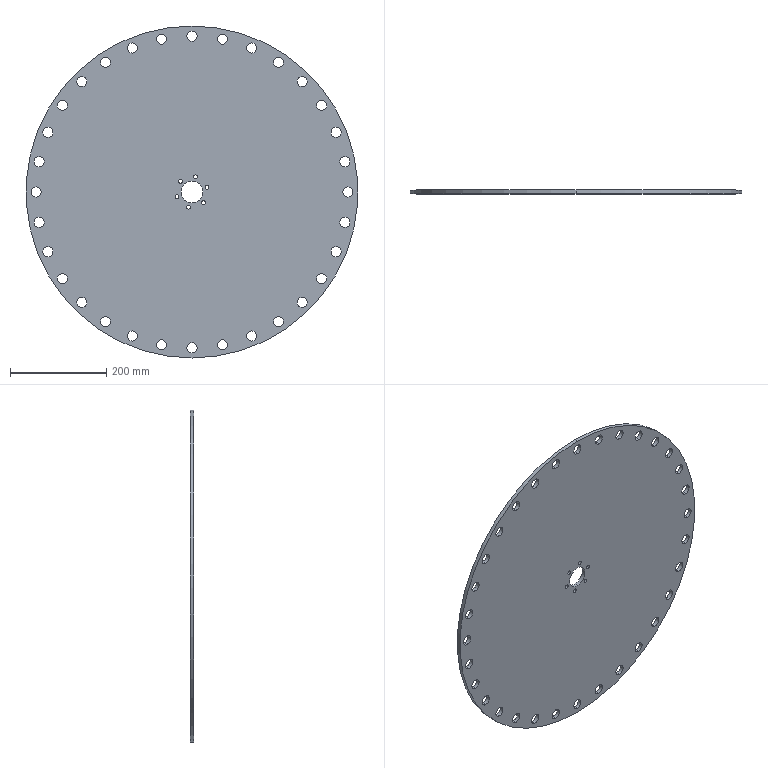Part | 1 solid | 82 faces | box 690 x 8 x 690 mm | volume 2887507 mm3 | cylinder 80 | plane 2 | commonest cylinder face diameters 21 x64 8 x12 45.2 x2 690 x2